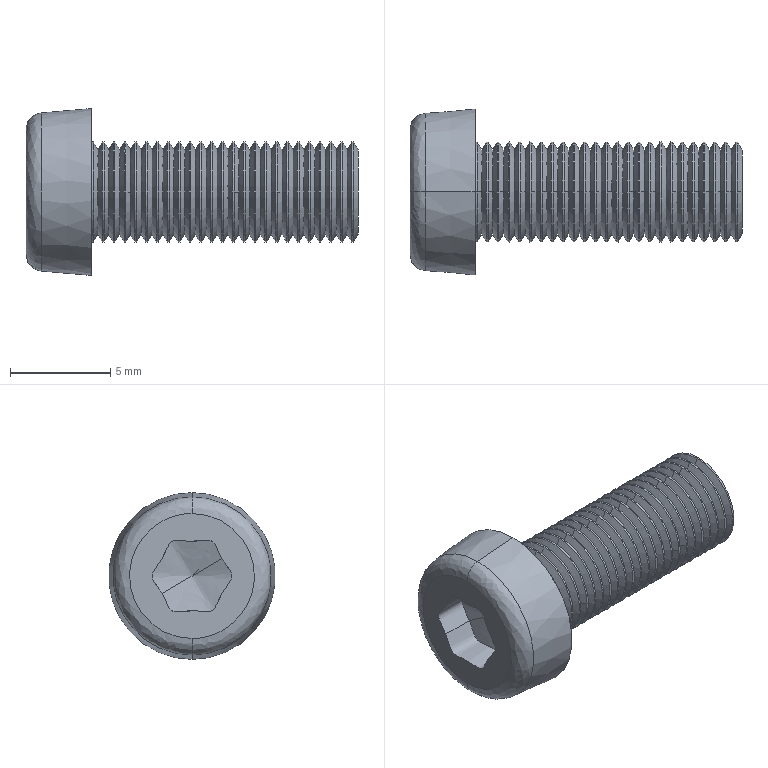Part | SolidWorks | features BaseBody 1, Scale 1 | 1 solid | 159 faces | box 16.583 x 8.333 x 8.333 mm | volume 372.356 mm3 | cone 100 | cylinder 50 | spline 6 | plane 3 | commonest cylinder face diameters 5 x50